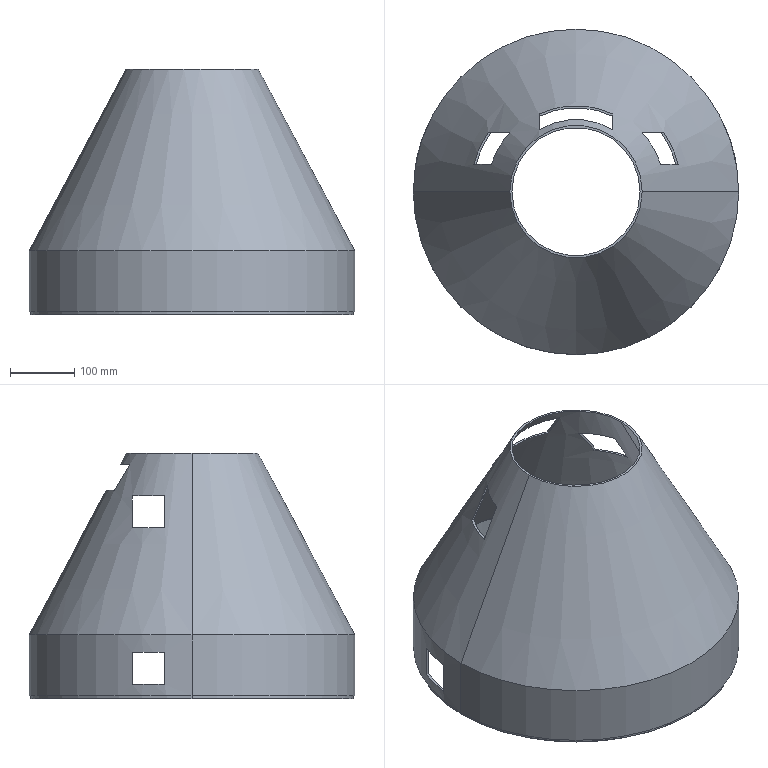Part | SolidWorks | features Cut 2, Extrusion 1, ICE 1, Revolution 1 | 1 solid | 34 faces | box 508 x 508 x 384 mm | volume 1629335 mm3 | plane 24 | cylinder 6 | cone 4 | commonest cylinder face diameters 500 x2 503 x2 508 x2
STEP:
#1=CARTESIAN_POINT('',(-251.5,0.,5.));
#2=VERTEX_POINT('',#1);
#3=CARTESIAN_POINT('',(251.5,0.,5.));
#4=VERTEX_POINT('',#3);
#5=CARTESIAN_POINT('',(0.,0.,5.));
#6=DIRECTION('',(0.,0.,-1.));
#7=DIRECTION('',(-1.,0.,0.));
#8=AXIS2_PLACEMENT_3D('',#5,#6,#7);
#9=CIRCLE('',#8,251.5);
#10=EDGE_CURVE('',#2,#4,#9,.T.);
#11=ORIENTED_EDGE('',*,*,#10,.T.);
#12=CARTESIAN_POINT('',(251.5,0.,0.));
#13=VERTEX_POINT('',#12);
#14=CARTESIAN_POINT('',(251.5,0.,5.));
#15=DIRECTION('',(0.,0.,-1.));
#16=VECTOR('',#15,1000.);
#17=LINE('',#14,#16);
#18=EDGE_CURVE('',#4,#13,#17,.T.);
#19=ORIENTED_EDGE('',*,*,#18,.T.);
#20=CARTESIAN_POINT('',(-251.5,0.,0.));
#21=VERTEX_POINT('',#20);
#22=CARTESIAN_POINT('',(0.,0.,0.));
#23=DIRECTION('',(0.,0.,-1.));
#24=DIRECTION('',(-1.,0.,0.));
#25=AXIS2_PLACEMENT_3D('',#22,#23,#24);
#26=CIRCLE('',#25,251.5);
#27=EDGE_CURVE('',#21,#13,#26,.T.);
#28=ORIENTED_EDGE('',*,*,#27,.F.);
#29=CARTESIAN_POINT('',(-251.5,0.,5.));
#30=DIRECTION('',(0.,0.,-1.));
#31=VECTOR('',#30,1000.);
#32=LINE('',#29,#31);
#33=EDGE_CURVE('',#2,#21,#32,.T.);
#34=ORIENTED_EDGE('',*,*,#33,.F.);
#35=EDGE_LOOP('',(#11,#19,#28,#34));
#36=FACE_OUTER_BOUND('',#35,.T.);
#37=CARTESIAN_POINT('',(0.,0.,5.));
#38=DIRECTION('',(0.,0.,-1.));
#39=DIRECTION('',(-1.,0.,0.));
#40=AXIS2_PLACEMENT_3D('',#37,#38,#39);
#41=CYLINDRICAL_SURFACE('',#40,251.5);
#42=ADVANCED_FACE('',(#36),#41,.T.);
#43=CARTESIAN_POINT('',(100.,0.,384.));
#44=VERTEX_POINT('',#43);
#45=CARTESIAN_POINT('',(-100.,0.,384.));
#46=VERTEX_POINT('',#45);
#47=CARTESIAN_POINT('',(0.,0.,384.));
#48=DIRECTION('',(0.,0.,-1.));
#49=DIRECTION('',(-1.,0.,0.));
#50=AXIS2_PLACEMENT_3D('',#47,#48,#49);
#51=CIRCLE('',#50,100.);
#52=EDGE_CURVE('',#44,#46,#51,.T.);
#53=ORIENTED_EDGE('',*,*,#52,.F.);
#54=CARTESIAN_POINT('',(250.604,0.,100.));
#55=VERTEX_POINT('',#54);
#56=CARTESIAN_POINT('',(250.604,0.,100.));
#57=DIRECTION('',(0.4685,0.,-0.8835));
#58=VECTOR('',#57,1000.);
#59=LINE('',#56,#58);
#60=EDGE_CURVE('',#44,#55,#59,.T.);
#61=ORIENTED_EDGE('',*,*,#60,.T.);
#62=CARTESIAN_POINT('',(-250.604,0.,100.));
#63=VERTEX_POINT('',#62);
#64=CARTESIAN_POINT('',(0.,0.,100.));
#65=DIRECTION('',(0.,0.,-1.));
#66=DIRECTION('',(-1.,0.,0.));
#67=AXIS2_PLACEMENT_3D('',#64,#65,#66);
#68=CIRCLE('',#67,250.604);
#69=EDGE_CURVE('',#55,#63,#68,.T.);
#70=ORIENTED_EDGE('',*,*,#69,.T.);
#71=CARTESIAN_POINT('',(-250.604,0.,100.));
#72=DIRECTION('',(-0.4685,0.,-0.8835));
#73=VECTOR('',#72,1000.);
#74=LINE('',#71,#73);
#75=EDGE_CURVE('',#46,#63,#74,.T.);
#76=ORIENTED_EDGE('',*,*,#75,.F.);
#77=EDGE_LOOP('',(#53,#61,#70,#76));
#78=FACE_OUTER_BOUND('',#77,.T.);
#79=CARTESIAN_POINT('',(0.,0.,100.));
#80=DIRECTION('',(0.,0.,-1.));
#81=DIRECTION('',(-1.,0.,0.));
#82=AXIS2_PLACEMENT_3D('',#79,#80,#81);
#83=CONICAL_SURFACE('',#82,250.604,0.4876);
#84=ADVANCED_FACE('',(#78),#83,.F.);
#85=CARTESIAN_POINT('',(57.407,96.803,366.747));
#86=VERTEX_POINT('',#85);
#87=CARTESIAN_POINT('',(-57.217,96.915,366.747));
#88=VERTEX_POINT('',#87);
#89=CARTESIAN_POINT('',(0.,0.,366.747));
#90=DIRECTION('',(0.,0.,1.));
#91=DIRECTION('',(0.,-1.,0.));
#92=AXIS2_PLACEMENT_3D('',#89,#90,#91);
#93=CIRCLE('',#92,112.545);
#94=EDGE_CURVE('',#86,#88,#93,.T.);
#95=ORIENTED_EDGE('',*,*,#94,.T.);
#96=CARTESIAN_POINT('',(-57.217,121.451,325.81));
#97=VERTEX_POINT('',#96);
#98=CARTESIAN_POINT('',(-57.217,96.915,366.747));
#99=CARTESIAN_POINT('',(-57.217,101.084,359.978));
#100=CARTESIAN_POINT('',(-57.217,105.204,353.175));
#101=CARTESIAN_POINT('',(-57.217,113.376,339.524));
#102=CARTESIAN_POINT('',(-57.217,117.427,332.674));
#103=CARTESIAN_POINT('',(-57.217,121.451,325.81));
#104=B_SPLINE_CURVE_WITH_KNOTS('',3,(#98,#99,#100,#101,#102,#103),.UNSPECIFIED.,.F.,.F.,(4,2,4),(0.4066,0.43,0.4535),.UNSPECIFIED.);
#105=EDGE_CURVE('',#88,#97,#104,.T.);
#106=ORIENTED_EDGE('',*,*,#105,.T.);
#107=CARTESIAN_POINT('',(57.407,121.361,325.81));
#108=VERTEX_POINT('',#107);
#109=CARTESIAN_POINT('',(0.,0.,325.81));
#110=DIRECTION('',(0.,0.,-1.));
#111=DIRECTION('',(0.,1.,0.));
#112=AXIS2_PLACEMENT_3D('',#109,#110,#111);
#113=CIRCLE('',#112,134.254);
#114=EDGE_CURVE('',#97,#108,#113,.T.);
#115=ORIENTED_EDGE('',*,*,#114,.T.);
#116=CARTESIAN_POINT('',(57.407,121.361,325.81));
#117=CARTESIAN_POINT('',(57.407,117.335,332.673));
#118=CARTESIAN_POINT('',(57.407,113.282,339.521));
#119=CARTESIAN_POINT('',(57.407,105.104,353.171));
#120=CARTESIAN_POINT('',(57.407,100.979,359.974));
#121=CARTESIAN_POINT('',(57.407,96.803,366.747));
#122=B_SPLINE_CURVE_WITH_KNOTS('',3,(#116,#117,#118,#119,#120,#121),.UNSPECIFIED.,.F.,.F.,(4,2,4),(0.1407,0.1646,0.1885),.UNSPECIFIED.);
#123=EDGE_CURVE('',#108,#86,#122,.T.);
#124=ORIENTED_EDGE('',*,*,#123,.T.);
#125=EDGE_LOOP('',(#95,#106,#115,#124));
#126=FACE_BOUND('',#125,.T.);
#127=CARTESIAN_POINT('',(159.672,42.9,267.2));
#128=VERTEX_POINT('',#127);
#129=CARTESIAN_POINT('',(132.024,42.9,317.2));
#130=VERTEX_POINT('',#129);
#131=CARTESIAN_POINT('',(159.672,42.9,267.2));
#132=CARTESIAN_POINT('',(150.505,42.9,283.893));
#133=CARTESIAN_POINT('',(141.3,42.9,300.566));
#134=CARTESIAN_POINT('',(132.024,42.9,317.2));
#135=B_SPLINE_CURVE_WITH_KNOTS('',3,(#131,#132,#133,#134),.UNSPECIFIED.,.F.,.F.,(4,4),(0.348,0.4051),.UNSPECIFIED.);
#136=EDGE_CURVE('',#128,#130,#135,.T.);
#137=ORIENTED_EDGE('',*,*,#136,.T.);
#138=CARTESIAN_POINT('',(103.153,92.9,317.2));
#139=VERTEX_POINT('',#138);
#140=CARTESIAN_POINT('',(0.,0.,317.2));
#141=DIRECTION('',(0.,0.,1.));
#142=DIRECTION('',(1.,0.,0.));
#143=AXIS2_PLACEMENT_3D('',#140,#141,#142);
#144=CIRCLE('',#143,138.82);
#145=EDGE_CURVE('',#130,#139,#144,.T.);
#146=ORIENTED_EDGE('',*,*,#145,.T.);
#147=CARTESIAN_POINT('',(136.766,92.9,267.2));
#148=VERTEX_POINT('',#147);
#149=CARTESIAN_POINT('',(103.153,92.9,317.2));
#150=CARTESIAN_POINT('',(108.982,92.9,309.031));
#151=CARTESIAN_POINT('',(114.668,92.9,300.759));
#152=CARTESIAN_POINT('',(125.848,92.9,284.074));
#153=CARTESIAN_POINT('',(131.342,92.9,275.662));
#154=CARTESIAN_POINT('',(136.766,92.9,267.2));
#155=B_SPLINE_CURVE_WITH_KNOTS('',3,(#149,#150,#151,#152,#153,#154),.UNSPECIFIED.,.F.,.F.,(4,2,4),(0.6909,0.7211,0.7513),.UNSPECIFIED.);
#156=EDGE_CURVE('',#139,#148,#155,.T.);
#157=ORIENTED_EDGE('',*,*,#156,.T.);
#158=CARTESIAN_POINT('',(0.,0.,267.2));
#159=DIRECTION('',(0.,0.,-1.));
#160=DIRECTION('',(-1.,0.,0.));
#161=AXIS2_PLACEMENT_3D('',#158,#159,#160);
#162=CIRCLE('',#161,165.334);
#163=EDGE_CURVE('',#148,#128,#162,.T.);
#164=ORIENTED_EDGE('',*,*,#163,.T.);
#165=EDGE_LOOP('',(#137,#146,#157,#164));
#166=FACE_BOUND('',#165,.T.);
#167=CARTESIAN_POINT('',(-136.766,92.9,267.2));
#168=VERTEX_POINT('',#167);
#169=CARTESIAN_POINT('',(-103.153,92.9,317.2));
#170=VERTEX_POINT('',#169);
#171=CARTESIAN_POINT('',(-136.766,92.9,267.2));
#172=CARTESIAN_POINT('',(-131.352,92.9,275.646));
#173=CARTESIAN_POINT('',(-125.865,92.9,284.05));
#174=CARTESIAN_POINT('',(-114.686,92.9,300.732));
#175=CARTESIAN_POINT('',(-108.996,92.9,309.012));
#176=CARTESIAN_POINT('',(-103.153,92.9,317.2));
#177=B_SPLINE_CURVE_WITH_KNOTS('',3,(#171,#172,#173,#174,#175,#176),.UNSPECIFIED.,.F.,.F.,(4,2,4),(0.354,0.384,0.4141),.UNSPECIFIED.);
#178=EDGE_CURVE('',#168,#170,#177,.T.);
#179=ORIENTED_EDGE('',*,*,#178,.T.);
#180=CARTESIAN_POINT('',(-132.024,42.9,317.2));
#181=VERTEX_POINT('',#180);
#182=CARTESIAN_POINT('',(0.,0.,317.2));
#183=DIRECTION('',(0.,0.,1.));
#184=DIRECTION('',(1.,0.,0.));
#185=AXIS2_PLACEMENT_3D('',#182,#183,#184);
#186=CIRCLE('',#185,138.82);
#187=EDGE_CURVE('',#170,#181,#186,.T.);
#188=ORIENTED_EDGE('',*,*,#187,.T.);
#189=CARTESIAN_POINT('',(-159.672,42.9,267.2));
#190=VERTEX_POINT('',#189);
#191=CARTESIAN_POINT('',(-132.024,42.9,317.2));
#192=CARTESIAN_POINT('',(-141.299,42.9,300.567));
#193=CARTESIAN_POINT('',(-150.505,42.9,283.895));
#194=CARTESIAN_POINT('',(-159.672,42.9,267.2));
#195=B_SPLINE_CURVE_WITH_KNOTS('',3,(#191,#192,#193,#194),.UNSPECIFIED.,.F.,.F.,(4,4),(0.8629,0.9203),.UNSPECIFIED.);
#196=EDGE_CURVE('',#181,#190,#195,.T.);
#197=ORIENTED_EDGE('',*,*,#196,.T.);
#198=CARTESIAN_POINT('',(0.,0.,267.2));
#199=DIRECTION('',(0.,0.,-1.));
#200=DIRECTION('',(-1.,0.,0.));
#201=AXIS2_PLACEMENT_3D('',#198,#199,#200);
#202=CIRCLE('',#201,165.334);
#203=EDGE_CURVE('',#190,#168,#202,.T.);
#204=ORIENTED_EDGE('',*,*,#203,.T.);
#205=EDGE_LOOP('',(#179,#188,#197,#204));
#206=FACE_BOUND('',#205,.T.);
#207=CARTESIAN_POINT('',(-103.396,0.,384.));
#208=VERTEX_POINT('',#207);
#209=CARTESIAN_POINT('',(103.396,0.,384.));
#210=VERTEX_POINT('',#209);
#211=CARTESIAN_POINT('',(0.,0.,384.));
#212=DIRECTION('',(0.,0.,-1.));
#213=DIRECTION('',(-1.,0.,0.));
#214=AXIS2_PLACEMENT_3D('',#211,#212,#213);
#215=CIRCLE('',#214,103.396);
#216=EDGE_CURVE('',#208,#210,#215,.T.);
#217=ORIENTED_EDGE('',*,*,#216,.T.);
#218=CARTESIAN_POINT('',(254.,0.,100.));
#219=VERTEX_POINT('',#218);
#220=CARTESIAN_POINT('',(103.396,0.,384.));
#221=DIRECTION('',(0.4685,0.,-0.8835));
#222=VECTOR('',#221,1000.);
#223=LINE('',#220,#222);
#224=EDGE_CURVE('',#210,#219,#223,.T.);
#225=ORIENTED_EDGE('',*,*,#224,.T.);
#226=CARTESIAN_POINT('',(-254.,0.,100.));
#227=VERTEX_POINT('',#226);
#228=CARTESIAN_POINT('',(0.,0.,100.));
#229=DIRECTION('',(0.,0.,1.));
#230=DIRECTION('',(1.,0.,0.));
#231=AXIS2_PLACEMENT_3D('',#228,#229,#230);
#232=CIRCLE('',#231,254.);
#233=EDGE_CURVE('',#219,#227,#232,.T.);
#234=ORIENTED_EDGE('',*,*,#233,.T.);
#235=CARTESIAN_POINT('',(-103.396,0.,384.));
#236=DIRECTION('',(-0.4685,0.,-0.8835));
#237=VECTOR('',#236,1000.);
#238=LINE('',#235,#237);
#239=EDGE_CURVE('',#208,#227,#238,.T.);
#240=ORIENTED_EDGE('',*,*,#239,.F.);
#241=EDGE_LOOP('',(#217,#225,#234,#240));
#242=FACE_OUTER_BOUND('',#241,.T.);
#243=CARTESIAN_POINT('',(0.,0.,384.));
#244=DIRECTION('',(0.,0.,-1.));
#245=DIRECTION('',(-1.,0.,0.));
#246=AXIS2_PLACEMENT_3D('',#243,#244,#245);
#247=CONICAL_SURFACE('',#246,103.396,0.4876);
#248=ADVANCED_FACE('',(#126,#166,#206,#242),#247,.T.);
#249=CARTESIAN_POINT('',(-250.,0.,100.));
#250=VERTEX_POINT('',#249);
#251=CARTESIAN_POINT('',(250.,0.,100.));
#252=VERTEX_POINT('',#251);
#253=CARTESIAN_POINT('',(0.,0.,100.));
#254=DIRECTION('',(0.,0.,1.));
#255=DIRECTION('',(1.,0.,0.));
#256=AXIS2_PLACEMENT_3D('',#253,#254,#255);
#257=CIRCLE('',#256,250.);
#258=EDGE_CURVE('',#250,#252,#257,.T.);
#259=ORIENTED_EDGE('',*,*,#258,.T.);
#260=CARTESIAN_POINT('',(250.,0.,0.));
#261=VERTEX_POINT('',#260);
#262=CARTESIAN_POINT('',(250.,0.,100.));
#263=DIRECTION('',(0.,0.,-1.));
#264=VECTOR('',#263,1000.);
#265=LINE('',#262,#264);
#266=EDGE_CURVE('',#252,#261,#265,.T.);
#267=ORIENTED_EDGE('',*,*,#266,.T.);
#268=CARTESIAN_POINT('',(-250.,0.,0.));
#269=VERTEX_POINT('',#268);
#270=CARTESIAN_POINT('',(0.,0.,0.));
#271=DIRECTION('',(0.,0.,1.));
#272=DIRECTION('',(1.,0.,0.));
#273=AXIS2_PLACEMENT_3D('',#270,#271,#272);
#274=CIRCLE('',#273,250.);
#275=EDGE_CURVE('',#269,#261,#274,.T.);
#276=ORIENTED_EDGE('',*,*,#275,.F.);
#277=CARTESIAN_POINT('',(-250.,0.,100.));
#278=DIRECTION('',(0.,0.,-1.));
#279=VECTOR('',#278,1000.);
#280=LINE('',#277,#279);
#281=EDGE_CURVE('',#250,#269,#280,.T.);
#282=ORIENTED_EDGE('',*,*,#281,.F.);
#283=EDGE_LOOP('',(#259,#267,#276,#282));
#284=FACE_OUTER_BOUND('',#283,.T.);
#285=CARTESIAN_POINT('',(0.,0.,100.));
#286=DIRECTION('',(0.,0.,-1.));
#287=DIRECTION('',(-1.,0.,0.));
#288=AXIS2_PLACEMENT_3D('',#285,#286,#287);
#289=CYLINDRICAL_SURFACE('',#288,250.);
#290=ADVANCED_FACE('',(#284),#289,.F.);
#291=CARTESIAN_POINT('',(250.351,42.9,22.8));
#292=VERTEX_POINT('',#291);
#293=CARTESIAN_POINT('',(250.351,42.9,72.8));
#294=VERTEX_POINT('',#293);
#295=CARTESIAN_POINT('',(250.351,42.9,100.));
#296=DIRECTION('',(0.,0.,1.));
#297=VECTOR('',#296,1000.);
#298=LINE('',#295,#297);
#299=EDGE_CURVE('',#292,#294,#298,.T.);
#300=ORIENTED_EDGE('',*,*,#299,.T.);
#301=CARTESIAN_POINT('',(236.401,92.9,72.8));
#302=VERTEX_POINT('',#301);
#303=CARTESIAN_POINT('',(0.,0.,72.8));
#304=DIRECTION('',(0.,0.,1.));
#305=DIRECTION('',(1.,0.,0.));
#306=AXIS2_PLACEMENT_3D('',#303,#304,#305);
#307=CIRCLE('',#306,254.);
#308=EDGE_CURVE('',#294,#302,#307,.T.);
#309=ORIENTED_EDGE('',*,*,#308,.T.);
#310=CARTESIAN_POINT('',(236.401,92.9,22.8));
#311=VERTEX_POINT('',#310);
#312=CARTESIAN_POINT('',(236.401,92.9,100.));
#313=DIRECTION('',(0.,0.,-1.));
#314=VECTOR('',#313,1000.);
#315=LINE('',#312,#314);
#316=EDGE_CURVE('',#302,#311,#315,.T.);
#317=ORIENTED_EDGE('',*,*,#316,.T.);
#318=CARTESIAN_POINT('',(0.,0.,22.8));
#319=DIRECTION('',(0.,0.,-1.));
#320=DIRECTION('',(-1.,0.,0.));
#321=AXIS2_PLACEMENT_3D('',#318,#319,#320);
#322=CIRCLE('',#321,254.);
#323=EDGE_CURVE('',#311,#292,#322,.T.);
#324=ORIENTED_EDGE('',*,*,#323,.T.);
#325=EDGE_LOOP('',(#300,#309,#317,#324));
#326=FACE_BOUND('',#325,.T.);
#327=CARTESIAN_POINT('',(-236.401,92.9,22.8));
#328=VERTEX_POINT('',#327);
#329=CARTESIAN_POINT('',(-236.401,92.9,72.8));
#330=VERTEX_POINT('',#329);
#331=CARTESIAN_POINT('',(-236.401,92.9,100.));
#332=DIRECTION('',(0.,0.,1.));
#333=VECTOR('',#332,1000.);
#334=LINE('',#331,#333);
#335=EDGE_CURVE('',#328,#330,#334,.T.);
#336=ORIENTED_EDGE('',*,*,#335,.T.);
#337=CARTESIAN_POINT('',(-250.351,42.9,72.8));
#338=VERTEX_POINT('',#337);
#339=CARTESIAN_POINT('',(0.,0.,72.8));
#340=DIRECTION('',(0.,0.,1.));
#341=DIRECTION('',(1.,0.,0.));
#342=AXIS2_PLACEMENT_3D('',#339,#340,#341);
#343=CIRCLE('',#342,254.);
#344=EDGE_CURVE('',#330,#338,#343,.T.);
#345=ORIENTED_EDGE('',*,*,#344,.T.);
#346=CARTESIAN_POINT('',(-250.351,42.9,22.8));
#347=VERTEX_POINT('',#346);
#348=CARTESIAN_POINT('',(-250.351,42.9,100.));
#349=DIRECTION('',(0.,0.,-1.));
#350=VECTOR('',#349,1000.);
#351=LINE('',#348,#350);
#352=EDGE_CURVE('',#338,#347,#351,.T.);
#353=ORIENTED_EDGE('',*,*,#352,.T.);
#354=CARTESIAN_POINT('',(0.,0.,22.8));
#355=DIRECTION('',(0.,0.,-1.));
#356=DIRECTION('',(-1.,0.,0.));
#357=AXIS2_PLACEMENT_3D('',#354,#355,#356);
#358=CIRCLE('',#357,254.);
#359=EDGE_CURVE('',#347,#328,#358,.T.);
#360=ORIENTED_EDGE('',*,*,#359,.T.);
#361=EDGE_LOOP('',(#336,#345,#353,#360));
#362=FACE_BOUND('',#361,.T.);
#363=ORIENTED_EDGE('',*,*,#233,.F.);
#364=CARTESIAN_POINT('',(254.,0.,5.));
#365=VERTEX_POINT('',#364);
#366=CARTESIAN_POINT('',(254.,0.,100.));
#367=DIRECTION('',(0.,0.,-1.));
#368=VECTOR('',#367,1000.);
#369=LINE('',#366,#368);
#370=EDGE_CURVE('',#219,#365,#369,.T.);
#371=ORIENTED_EDGE('',*,*,#370,.T.);
#372=CARTESIAN_POINT('',(-254.,0.,5.));
#373=VERTEX_POINT('',#372);
#374=CARTESIAN_POINT('',(0.,0.,5.));
#375=DIRECTION('',(0.,0.,-1.));
#376=DIRECTION('',(-1.,0.,0.));
#377=AXIS2_PLACEMENT_3D('',#374,#375,#376);
#378=CIRCLE('',#377,254.);
#379=EDGE_CURVE('',#373,#365,#378,.T.);
#380=ORIENTED_EDGE('',*,*,#379,.F.);
#381=CARTESIAN_POINT('',(-254.,0.,100.));
#382=DIRECTION('',(0.,0.,-1.));
#383=VECTOR('',#382,1000.);
#384=LINE('',#381,#383);
#385=EDGE_CURVE('',#227,#373,#384,.T.);
#386=ORIENTED_EDGE('',*,*,#385,.F.);
#387=EDGE_LOOP('',(#363,#371,#380,#386));
#388=FACE_OUTER_BOUND('',#387,.T.);
#389=CARTESIAN_POINT('',(0.,0.,100.));
#390=DIRECTION('',(0.,0.,-1.));
#391=DIRECTION('',(-1.,0.,0.));
#392=AXIS2_PLACEMENT_3D('',#389,#390,#391);
#393=CYLINDRICAL_SURFACE('',#392,254.);
#394=ADVANCED_FACE('',(#326,#362,#388),#393,.T.);
#395=ORIENTED_EDGE('',*,*,#275,.T.);
#396=CARTESIAN_POINT('',(0.,0.,0.));
#397=DIRECTION('',(0.,0.,1.));
#398=DIRECTION('',(1.,0.,0.));
#399=AXIS2_PLACEMENT_3D('',#396,#397,#398);
#400=CIRCLE('',#399,250.);
#401=EDGE_CURVE('',#261,#269,#400,.T.);
#402=ORIENTED_EDGE('',*,*,#401,.T.);
#403=EDGE_LOOP('',(#395,#402));
#404=FACE_BOUND('',#403,.T.);
#405=ORIENTED_EDGE('',*,*,#27,.T.);
#406=CARTESIAN_POINT('',(0.,0.,0.));
#407=DIRECTION('',(0.,0.,-1.));
#408=DIRECTION('',(-1.,0.,0.));
#409=AXIS2_PLACEMENT_3D('',#406,#407,#408);
#410=CIRCLE('',#409,251.5);
#411=EDGE_CURVE('',#13,#21,#410,.T.);
#412=ORIENTED_EDGE('',*,*,#411,.T.);
#413=EDGE_LOOP('',(#405,#412));
#414=FACE_OUTER_BOUND('',#413,.T.);
#415=CARTESIAN_POINT('',(0.,0.,0.));
#416=DIRECTION('',(0.,0.,1.));
#417=DIRECTION('',(1.,0.,0.));
#418=AXIS2_PLACEMENT_3D('',#415,#416,#417);
#419=PLANE('',#418);
#420=ADVANCED_FACE('',(#404,#414),#419,.F.);
#421=ORIENTED_EDGE('',*,*,#370,.F.);
#422=CARTESIAN_POINT('',(0.,0.,100.));
#423=DIRECTION('',(0.,0.,1.));
#424=DIRECTION('',(1.,0.,0.));
#425=AXIS2_PLACEMENT_3D('',#422,#423,#424);
#426=CIRCLE('',#425,254.);
#427=EDGE_CURVE('',#227,#219,#426,.T.);
#428=ORIENTED_EDGE('',*,*,#427,.F.);
#429=ORIENTED_EDGE('',*,*,#385,.T.);
#430=CARTESIAN_POINT('',(0.,0.,5.));
#431=DIRECTION('',(0.,0.,-1.));
#432=DIRECTION('',(-1.,0.,0.));
#433=AXIS2_PLACEMENT_3D('',#430,#431,#432);
#434=CIRCLE('',#433,254.);
#435=EDGE_CURVE('',#365,#373,#434,.T.);
#436=ORIENTED_EDGE('',*,*,#435,.F.);
#437=EDGE_LOOP('',(#421,#428,#429,#436));
#438=FACE_OUTER_BOUND('',#437,.T.);
#439=CARTESIAN_POINT('',(0.,0.,100.));
#440=DIRECTION('',(0.,0.,-1.));
#441=DIRECTION('',(-1.,0.,0.));
#442=AXIS2_PLACEMENT_3D('',#439,#440,#441);
#443=CYLINDRICAL_SURFACE('',#442,254.);
#444=ADVANCED_FACE('',(#438),#443,.T.);
#445=ORIENTED_EDGE('',*,*,#258,.F.);
#446=CARTESIAN_POINT('',(0.,0.,100.));
#447=DIRECTION('',(0.,0.,1.));
#448=DIRECTION('',(1.,0.,0.));
#449=AXIS2_PLACEMENT_3D('',#446,#447,#448);
#450=CIRCLE('',#449,250.);
#451=EDGE_CURVE('',#252,#250,#450,.T.);
#452=ORIENTED_EDGE('',*,*,#451,.F.);
#453=EDGE_LOOP('',(#445,#452));
#454=FACE_BOUND('',#453,.T.);
#455=CARTESIAN_POINT('',(0.,0.,100.));
#456=DIRECTION('',(0.,0.,-1.));
#457=DIRECTION('',(-1.,0.,0.));
#458=AXIS2_PLACEMENT_3D('',#455,#456,#457);
#459=CIRCLE('',#458,250.604);
#460=EDGE_CURVE('',#63,#55,#459,.T.);
#461=ORIENTED_EDGE('',*,*,#460,.F.);
#462=ORIENTED_EDGE('',*,*,#69,.F.);
#463=EDGE_LOOP('',(#461,#462));
#464=FACE_OUTER_BOUND('',#463,.T.);
#465=CARTESIAN_POINT('',(0.,0.,100.));
#466=DIRECTION('',(0.,0.,1.));
#467=DIRECTION('',(1.,0.,0.));
#468=AXIS2_PLACEMENT_3D('',#465,#466,#467);
#469=PLANE('',#468);
#470=ADVANCED_FACE('',(#454,#464),#469,.T.);
#471=ORIENTED_EDGE('',*,*,#266,.F.);
#472=ORIENTED_EDGE('',*,*,#451,.T.);
#473=ORIENTED_EDGE('',*,*,#281,.T.);
#474=ORIENTED_EDGE('',*,*,#401,.F.);
#475=EDGE_LOOP('',(#471,#472,#473,#474));
#476=FACE_OUTER_BOUND('',#475,.T.);
#477=CARTESIAN_POINT('',(-232.098,92.9,72.8));
#478=VERTEX_POINT('',#477);
#479=CARTESIAN_POINT('',(-246.292,42.9,72.8));
#480=VERTEX_POINT('',#479);
#481=CARTESIAN_POINT('',(0.,0.,72.8));
#482=DIRECTION('',(0.,0.,1.));
#483=DIRECTION('',(1.,0.,0.));
#484=AXIS2_PLACEMENT_3D('',#481,#482,#483);
#485=CIRCLE('',#484,250.);
#486=EDGE_CURVE('',#478,#480,#485,.T.);
#487=ORIENTED_EDGE('',*,*,#486,.F.);
#488=CARTESIAN_POINT('',(-232.098,92.9,22.8));
#489=VERTEX_POINT('',#488);
#490=CARTESIAN_POINT('',(-232.098,92.9,100.));
#491=DIRECTION('',(0.,0.,1.));
#492=VECTOR('',#491,1000.);
#493=LINE('',#490,#492);
#494=EDGE_CURVE('',#489,#478,#493,.T.);
#495=ORIENTED_EDGE('',*,*,#494,.F.);
#496=CARTESIAN_POINT('',(-246.292,42.9,22.8));
#497=VERTEX_POINT('',#496);
#498=CARTESIAN_POINT('',(0.,0.,22.8));
#499=DIRECTION('',(0.,0.,-1.));
#500=DIRECTION('',(-1.,0.,0.));
#501=AXIS2_PLACEMENT_3D('',#498,#499,#500);
#502=CIRCLE('',#501,250.);
#503=EDGE_CURVE('',#497,#489,#502,.T.);
#504=ORIENTED_EDGE('',*,*,#503,.F.);
#505=CARTESIAN_POINT('',(-246.292,42.9,100.));
#506=DIRECTION('',(0.,0.,-1.));
#507=VECTOR('',#506,1000.);
#508=LINE('',#505,#507);
#509=EDGE_CURVE('',#480,#497,#508,.T.);
#510=ORIENTED_EDGE('',*,*,#509,.F.);
#511=EDGE_LOOP('',(#487,#495,#504,#510));
#512=FACE_BOUND('',#511,.T.);
#513=CARTESIAN_POINT('',(246.292,42.9,72.8));
#514=VERTEX_POINT('',#513);
#515=CARTESIAN_POINT('',(232.098,92.9,72.8));
#516=VERTEX_POINT('',#515);
#517=CARTESIAN_POINT('',(0.,0.,72.8));
#518=DIRECTION('',(0.,0.,1.));
#519=DIRECTION('',(1.,0.,0.));
#520=AXIS2_PLACEMENT_3D('',#517,#518,#519);
#521=CIRCLE('',#520,250.);
#522=EDGE_CURVE('',#514,#516,#521,.T.);
#523=ORIENTED_EDGE('',*,*,#522,.F.);
#524=CARTESIAN_POINT('',(246.292,42.9,22.8));
#525=VERTEX_POINT('',#524);
#526=CARTESIAN_POINT('',(246.292,42.9,100.));
#527=DIRECTION('',(0.,0.,1.));
#528=VECTOR('',#527,1000.);
#529=LINE('',#526,#528);
#530=EDGE_CURVE('',#525,#514,#529,.T.);
#531=ORIENTED_EDGE('',*,*,#530,.F.);
#532=CARTESIAN_POINT('',(232.098,92.9,22.8));
#533=VERTEX_POINT('',#532);
#534=CARTESIAN_POINT('',(0.,0.,22.8));
#535=DIRECTION('',(0.,0.,-1.));
#536=DIRECTION('',(-1.,0.,0.));
#537=AXIS2_PLACEMENT_3D('',#534,#535,#536);
#538=CIRCLE('',#537,250.);
#539=EDGE_CURVE('',#533,#525,#538,.T.);
#540=ORIENTED_EDGE('',*,*,#539,.F.);
#541=CARTESIAN_POINT('',(232.098,92.9,100.));
#542=DIRECTION('',(0.,0.,-1.));
#543=VECTOR('',#542,1000.);
#544=LINE('',#541,#543);
#545=EDGE_CURVE('',#516,#533,#544,.T.);
#546=ORIENTED_EDGE('',*,*,#545,.F.);
#547=EDGE_LOOP('',(#523,#531,#540,#546));
#548=FACE_BOUND('',#547,.T.);
#549=CARTESIAN_POINT('',(0.,0.,100.));
#550=DIRECTION('',(0.,0.,-1.));
#551=DIRECTION('',(-1.,0.,0.));
#552=AXIS2_PLACEMENT_3D('',#549,#550,#551);
#553=CYLINDRICAL_SURFACE('',#552,250.);
#554=ADVANCED_FACE('',(#476,#512,#548),#553,.F.);
#555=ORIENTED_EDGE('',*,*,#224,.F.);
#556=CARTESIAN_POINT('',(0.,0.,384.));
#557=DIRECTION('',(0.,0.,-1.));
#558=DIRECTION('',(-1.,0.,0.));
#559=AXIS2_PLACEMENT_3D('',#556,#557,#558);
#560=CIRCLE('',#559,103.396);
#561=EDGE_CURVE('',#210,#208,#560,.T.);
#562=ORIENTED_EDGE('',*,*,#561,.T.);
#563=ORIENTED_EDGE('',*,*,#239,.T.);
#564=ORIENTED_EDGE('',*,*,#427,.T.);
#565=EDGE_LOOP('',(#555,#562,#563,#564));
#566=FACE_OUTER_BOUND('',#565,.T.);
#567=CARTESIAN_POINT('',(0.,0.,384.));
#568=DIRECTION('',(0.,0.,-1.));
#569=DIRECTION('',(-1.,0.,0.));
#570=AXIS2_PLACEMENT_3D('',#567,#568,#569);
#571=CONICAL_SURFACE('',#570,103.396,0.4876);
#572=ADVANCED_FACE('',(#566),#571,.T.);
#573=ORIENTED_EDGE('',*,*,#216,.F.);
#574=ORIENTED_EDGE('',*,*,#561,.F.);
#575=EDGE_LOOP('',(#573,#574));
#576=FACE_OUTER_BOUND('',#575,.T.);
#577=CARTESIAN_POINT('',(0.,0.,384.));
#578=DIRECTION('',(0.,0.,-1.));
#579=DIRECTION('',(-1.,0.,0.));
#580=AXIS2_PLACEMENT_3D('',#577,#578,#579);
#581=CIRCLE('',#580,100.);
#582=EDGE_CURVE('',#46,#44,#581,.T.);
#583=ORIENTED_EDGE('',*,*,#582,.T.);
#584=ORIENTED_EDGE('',*,*,#52,.T.);
#585=EDGE_LOOP('',(#583,#584));
#586=FACE_BOUND('',#585,.T.);
#587=CARTESIAN_POINT('',(100.,0.,384.));
#588=DIRECTION('',(0.,0.,-1.));
#589=DIRECTION('',(-1.,0.,0.));
#590=AXIS2_PLACEMENT_3D('',#587,#588,#589);
#591=PLANE('',#590);
#592=ADVANCED_FACE('',(#576,#586),#591,.F.);
#593=ORIENTED_EDGE('',*,*,#60,.F.);
#594=ORIENTED_EDGE('',*,*,#582,.F.);
#595=ORIENTED_EDGE('',*,*,#75,.T.);
#596=ORIENTED_EDGE('',*,*,#460,.T.);
#597=EDGE_LOOP('',(#593,#594,#595,#596));
#598=FACE_OUTER_BOUND('',#597,.T.);
#599=CARTESIAN_POINT('',(57.407,117.594,325.81));
#600=VERTEX_POINT('',#599);
#601=CARTESIAN_POINT('',(-57.217,117.686,325.81));
#602=VERTEX_POINT('',#601);
#603=CARTESIAN_POINT('',(0.,0.,325.81));
#604=DIRECTION('',(0.,0.,1.));
#605=DIRECTION('',(0.,1.,0.));
#606=AXIS2_PLACEMENT_3D('',#603,#604,#605);
#607=CIRCLE('',#606,130.858);
#608=EDGE_CURVE('',#600,#602,#607,.T.);
#609=ORIENTED_EDGE('',*,*,#608,.T.);
#610=CARTESIAN_POINT('',(-57.217,92.95,366.747));
#611=VERTEX_POINT('',#610);
#612=CARTESIAN_POINT('',(-57.217,117.686,325.81));
#613=CARTESIAN_POINT('',(-57.217,113.637,332.678));
#614=CARTESIAN_POINT('',(-57.217,109.558,339.527));
#615=CARTESIAN_POINT('',(-57.217,101.322,353.178));
#616=CARTESIAN_POINT('',(-57.217,97.164,359.98));
#617=CARTESIAN_POINT('',(-57.217,92.95,366.747));
#618=B_SPLINE_CURVE_WITH_KNOTS('',3,(#612,#613,#614,#615,#616,#617),.UNSPECIFIED.,.F.,.F.,(4,2,4),(0.1408,0.1647,0.1886),.UNSPECIFIED.);
#619=EDGE_CURVE('',#602,#611,#618,.T.);
#620=ORIENTED_EDGE('',*,*,#619,.T.);
#621=CARTESIAN_POINT('',(57.407,92.833,366.747));
#622=VERTEX_POINT('',#621);
#623=CARTESIAN_POINT('',(0.,0.,366.747));
#624=DIRECTION('',(0.,0.,-1.));
#625=DIRECTION('',(0.,-1.,0.));
#626=AXIS2_PLACEMENT_3D('',#623,#624,#625);
#627=CIRCLE('',#626,109.149);
#628=EDGE_CURVE('',#611,#622,#627,.T.);
#629=ORIENTED_EDGE('',*,*,#628,.T.);
#630=CARTESIAN_POINT('',(57.407,92.833,366.747));
#631=CARTESIAN_POINT('',(57.407,97.05,359.985));
#632=CARTESIAN_POINT('',(57.407,101.211,353.185));
#633=CARTESIAN_POINT('',(57.407,109.455,339.533));
#634=CARTESIAN_POINT('',(57.407,113.539,332.681));
#635=CARTESIAN_POINT('',(57.407,117.594,325.81));
#636=B_SPLINE_CURVE_WITH_KNOTS('',3,(#630,#631,#632,#633,#634,#635),.UNSPECIFIED.,.F.,.F.,(4,2,4),(0.3985,0.422,0.4456),.UNSPECIFIED.);
#637=EDGE_CURVE('',#622,#600,#636,.T.);
#638=ORIENTED_EDGE('',*,*,#637,.T.);
#639=EDGE_LOOP('',(#609,#620,#629,#638));
#640=FACE_BOUND('',#639,.T.);
#641=CARTESIAN_POINT('',(-156.153,42.9,267.2));
#642=VERTEX_POINT('',#641);
#643=CARTESIAN_POINT('',(-128.449,42.9,317.2));
#644=VERTEX_POINT('',#643);
#645=CARTESIAN_POINT('',(-156.153,42.9,267.2));
#646=CARTESIAN_POINT('',(-146.971,42.9,283.895));
#647=CARTESIAN_POINT('',(-137.748,42.9,300.568));
#648=CARTESIAN_POINT('',(-128.449,42.9,317.2));
#649=B_SPLINE_CURVE_WITH_KNOTS('',3,(#645,#646,#647,#648),.UNSPECIFIED.,.F.,.F.,(4,4),(0.3435,0.4006),.UNSPECIFIED.);
#650=EDGE_CURVE('',#642,#644,#649,.T.);
#651=ORIENTED_EDGE('',*,*,#650,.T.);
#652=CARTESIAN_POINT('',(-98.535,92.9,317.2));
#653=VERTEX_POINT('',#652);
#654=CARTESIAN_POINT('',(0.,0.,317.2));
#655=DIRECTION('',(0.,0.,-1.));
#656=DIRECTION('',(1.,0.,0.));
#657=AXIS2_PLACEMENT_3D('',#654,#655,#656);
#658=CIRCLE('',#657,135.424);
#659=EDGE_CURVE('',#644,#653,#658,.T.);
#660=ORIENTED_EDGE('',*,*,#659,.T.);
#661=CARTESIAN_POINT('',(-132.641,92.9,267.2));
#662=VERTEX_POINT('',#661);
#663=CARTESIAN_POINT('',(-98.535,92.9,317.2));
#664=CARTESIAN_POINT('',(-104.489,92.9,309.031));
#665=CARTESIAN_POINT('',(-110.27,92.9,300.757));
#666=CARTESIAN_POINT('',(-121.609,92.9,284.072));
#667=CARTESIAN_POINT('',(-127.164,92.9,275.66));
#668=CARTESIAN_POINT('',(-132.641,92.9,267.2));
#669=B_SPLINE_CURVE_WITH_KNOTS('',3,(#663,#664,#665,#666,#667,#668),.UNSPECIFIED.,.F.,.F.,(4,2,4),(0.6709,0.7012,0.7315),.UNSPECIFIED.);
#670=EDGE_CURVE('',#653,#662,#669,.T.);
#671=ORIENTED_EDGE('',*,*,#670,.T.);
#672=CARTESIAN_POINT('',(0.,0.,267.2));
#673=DIRECTION('',(0.,0.,1.));
#674=DIRECTION('',(-1.,0.,0.));
#675=AXIS2_PLACEMENT_3D('',#672,#673,#674);
#676=CIRCLE('',#675,161.939);
#677=EDGE_CURVE('',#662,#642,#676,.T.);
#678=ORIENTED_EDGE('',*,*,#677,.T.);
#679=EDGE_LOOP('',(#651,#660,#671,#678));
#680=FACE_BOUND('',#679,.T.);
#681=CARTESIAN_POINT('',(132.641,92.9,267.2));
#682=VERTEX_POINT('',#681);
#683=CARTESIAN_POINT('',(98.535,92.9,317.2));
#684=VERTEX_POINT('',#683);
#685=CARTESIAN_POINT('',(132.641,92.9,267.2));
#686=CARTESIAN_POINT('',(127.165,92.9,275.659));
#687=CARTESIAN_POINT('',(121.609,92.9,284.071));
#688=CARTESIAN_POINT('',(110.271,92.9,300.756));
#689=CARTESIAN_POINT('',(104.489,92.9,309.03));
#690=CARTESIAN_POINT('',(98.535,92.9,317.2));
#691=B_SPLINE_CURVE_WITH_KNOTS('',3,(#685,#686,#687,#688,#689,#690),.UNSPECIFIED.,.F.,.F.,(4,2,4),(0.3496,0.3798,0.4101),.UNSPECIFIED.);
#692=EDGE_CURVE('',#682,#684,#691,.T.);
#693=ORIENTED_EDGE('',*,*,#692,.T.);
#694=CARTESIAN_POINT('',(128.449,42.9,317.2));
#695=VERTEX_POINT('',#694);
#696=CARTESIAN_POINT('',(0.,0.,317.2));
#697=DIRECTION('',(0.,0.,-1.));
#698=DIRECTION('',(1.,0.,0.));
#699=AXIS2_PLACEMENT_3D('',#696,#697,#698);
#700=CIRCLE('',#699,135.424);
#701=EDGE_CURVE('',#684,#695,#700,.T.);
#702=ORIENTED_EDGE('',*,*,#701,.T.);
#703=CARTESIAN_POINT('',(156.153,42.9,267.2));
#704=VERTEX_POINT('',#703);
#705=CARTESIAN_POINT('',(128.449,42.9,317.2));
#706=CARTESIAN_POINT('',(137.747,42.9,300.57));
#707=CARTESIAN_POINT('',(146.971,42.9,283.897));
#708=CARTESIAN_POINT('',(156.153,42.9,267.2));
#709=B_SPLINE_CURVE_WITH_KNOTS('',3,(#705,#706,#707,#708),.UNSPECIFIED.,.F.,.F.,(4,4),(0.8436,0.9011),.UNSPECIFIED.);
#710=EDGE_CURVE('',#695,#704,#709,.T.);
#711=ORIENTED_EDGE('',*,*,#710,.T.);
#712=CARTESIAN_POINT('',(0.,0.,267.2));
#713=DIRECTION('',(0.,0.,1.));
#714=DIRECTION('',(-1.,0.,0.));
#715=AXIS2_PLACEMENT_3D('',#712,#713,#714);
#716=CIRCLE('',#715,161.939);
#717=EDGE_CURVE('',#704,#682,#716,.T.);
#718=ORIENTED_EDGE('',*,*,#717,.T.);
#719=EDGE_LOOP('',(#693,#702,#711,#718));
#720=FACE_BOUND('',#719,.T.);
#721=CARTESIAN_POINT('',(0.,0.,100.));
#722=DIRECTION('',(0.,0.,-1.));
#723=DIRECTION('',(-1.,0.,0.));
#724=AXIS2_PLACEMENT_3D('',#721,#722,#723);
#725=CONICAL_SURFACE('',#724,250.604,0.4876);
#726=ADVANCED_FACE('',(#598,#640,#680,#720),#725,.F.);
#727=CARTESIAN_POINT('',(-500.,42.9,22.8));
#728=DIRECTION('',(1.,0.,0.));
#729=VECTOR('',#728,1000.);
#730=LINE('',#727,#729);
#731=EDGE_CURVE('',#525,#292,#730,.T.);
#732=ORIENTED_EDGE('',*,*,#731,.F.);
#733=ORIENTED_EDGE('',*,*,#530,.T.);
#734=CARTESIAN_POINT('',(-500.,42.9,72.8));
#735=DIRECTION('',(1.,0.,0.));
#736=VECTOR('',#735,1000.);
#737=LINE('',#734,#736);
#738=EDGE_CURVE('',#514,#294,#737,.T.);
#739=ORIENTED_EDGE('',*,*,#738,.T.);
#740=ORIENTED_EDGE('',*,*,#299,.F.);
#741=EDGE_LOOP('',(#732,#733,#739,#740));
#742=FACE_OUTER_BOUND('',#741,.T.);
#743=CARTESIAN_POINT('',(-500.,42.9,72.8));
#744=DIRECTION('',(0.,-1.,0.));
#745=DIRECTION('',(0.,0.,-1.));
#746=AXIS2_PLACEMENT_3D('',#743,#744,#745);
#747=PLANE('',#746);
#748=ADVANCED_FACE('',(#742),#747,.F.);
#749=CARTESIAN_POINT('',(-500.,92.9,22.8));
#750=DIRECTION('',(1.,0.,0.));
#751=VECTOR('',#750,1000.);
#752=LINE('',#749,#751);
#753=EDGE_CURVE('',#533,#311,#752,.T.);
#754=ORIENTED_EDGE('',*,*,#753,.F.);
#755=ORIENTED_EDGE('',*,*,#539,.T.);
#756=ORIENTED_EDGE('',*,*,#731,.T.);
#757=ORIENTED_EDGE('',*,*,#323,.F.);
#758=EDGE_LOOP('',(#754,#755,#756,#757));
#759=FACE_OUTER_BOUND('',#758,.T.);
#760=CARTESIAN_POINT('',(-500.,92.9,22.8));
#761=DIRECTION('',(0.,0.,-1.));
#762=DIRECTION('',(-1.,0.,0.));
#763=AXIS2_PLACEMENT_3D('',#760,#761,#762);
#764=PLANE('',#763);
#765=ADVANCED_FACE('',(#759),#764,.F.);
#766=CARTESIAN_POINT('',(-500.,92.9,72.8));
#767=DIRECTION('',(1.,0.,0.));
#768=VECTOR('',#767,1000.);
#769=LINE('',#766,#768);
#770=EDGE_CURVE('',#516,#302,#769,.T.);
#771=ORIENTED_EDGE('',*,*,#770,.F.);
#772=ORIENTED_EDGE('',*,*,#545,.T.);
#773=ORIENTED_EDGE('',*,*,#753,.T.);
#774=ORIENTED_EDGE('',*,*,#316,.F.);
#775=EDGE_LOOP('',(#771,#772,#773,#774));
#776=FACE_OUTER_BOUND('',#775,.T.);
#777=CARTESIAN_POINT('',(-500.,92.9,72.8));
#778=DIRECTION('',(0.,1.,0.));
#779=DIRECTION('',(0.,0.,1.));
#780=AXIS2_PLACEMENT_3D('',#777,#778,#779);
#781=PLANE('',#780);
#782=ADVANCED_FACE('',(#776),#781,.F.);
#783=ORIENTED_EDGE('',*,*,#738,.F.);
#784=ORIENTED_EDGE('',*,*,#522,.T.);
#785=ORIENTED_EDGE('',*,*,#770,.T.);
#786=ORIENTED_EDGE('',*,*,#308,.F.);
#787=EDGE_LOOP('',(#783,#784,#785,#786));
#788=FACE_OUTER_BOUND('',#787,.T.);
#789=CARTESIAN_POINT('',(-500.,92.9,72.8));
#790=DIRECTION('',(0.,0.,1.));
#791=DIRECTION('',(1.,0.,0.));
#792=AXIS2_PLACEMENT_3D('',#789,#790,#791);
#793=PLANE('',#792);
#794=ADVANCED_FACE('',(#788),#793,.F.);
#795=CARTESIAN_POINT('',(-500.,92.9,72.8));
#796=DIRECTION('',(1.,0.,0.));
#797=VECTOR('',#796,1000.);
#798=LINE('',#795,#797);
#799=EDGE_CURVE('',#330,#478,#798,.T.);
#800=ORIENTED_EDGE('',*,*,#799,.T.);
#801=ORIENTED_EDGE('',*,*,#486,.T.);
#802=CARTESIAN_POINT('',(-500.,42.9,72.8));
#803=DIRECTION('',(1.,0.,0.));
#804=VECTOR('',#803,1000.);
#805=LINE('',#802,#804);
#806=EDGE_CURVE('',#338,#480,#805,.T.);
#807=ORIENTED_EDGE('',*,*,#806,.F.);
#808=ORIENTED_EDGE('',*,*,#344,.F.);
#809=EDGE_LOOP('',(#800,#801,#807,#808));
#810=FACE_OUTER_BOUND('',#809,.T.);
#811=CARTESIAN_POINT('',(-500.,92.9,72.8));
#812=DIRECTION('',(0.,0.,1.));
#813=DIRECTION('',(1.,0.,0.));
#814=AXIS2_PLACEMENT_3D('',#811,#812,#813);
#815=PLANE('',#814);
#816=ADVANCED_FACE('',(#810),#815,.F.);
#817=CARTESIAN_POINT('',(-500.,92.9,22.8));
#818=DIRECTION('',(1.,0.,0.));
#819=VECTOR('',#818,1000.);
#820=LINE('',#817,#819);
#821=EDGE_CURVE('',#328,#489,#820,.T.);
#822=ORIENTED_EDGE('',*,*,#821,.T.);
#823=ORIENTED_EDGE('',*,*,#494,.T.);
#824=ORIENTED_EDGE('',*,*,#799,.F.);
#825=ORIENTED_EDGE('',*,*,#335,.F.);
#826=EDGE_LOOP('',(#822,#823,#824,#825));
#827=FACE_OUTER_BOUND('',#826,.T.);
#828=CARTESIAN_POINT('',(-500.,92.9,72.8));
#829=DIRECTION('',(0.,1.,0.));
#830=DIRECTION('',(0.,0.,1.));
#831=AXIS2_PLACEMENT_3D('',#828,#829,#830);
#832=PLANE('',#831);
#833=ADVANCED_FACE('',(#827),#832,.F.);
#834=CARTESIAN_POINT('',(-500.,42.9,22.8));
#835=DIRECTION('',(1.,0.,0.));
#836=VECTOR('',#835,1000.);
#837=LINE('',#834,#836);
#838=EDGE_CURVE('',#347,#497,#837,.T.);
#839=ORIENTED_EDGE('',*,*,#838,.T.);
#840=ORIENTED_EDGE('',*,*,#503,.T.);
#841=ORIENTED_EDGE('',*,*,#821,.F.);
#842=ORIENTED_EDGE('',*,*,#359,.F.);
#843=EDGE_LOOP('',(#839,#840,#841,#842));
#844=FACE_OUTER_BOUND('',#843,.T.);
#845=CARTESIAN_POINT('',(-500.,92.9,22.8));
#846=DIRECTION('',(0.,0.,-1.));
#847=DIRECTION('',(-1.,0.,0.));
#848=AXIS2_PLACEMENT_3D('',#845,#846,#847);
#849=PLANE('',#848);
#850=ADVANCED_FACE('',(#844),#849,.F.);
#851=ORIENTED_EDGE('',*,*,#806,.T.);
#852=ORIENTED_EDGE('',*,*,#509,.T.);
#853=ORIENTED_EDGE('',*,*,#838,.F.);
#854=ORIENTED_EDGE('',*,*,#352,.F.);
#855=EDGE_LOOP('',(#851,#852,#853,#854));
#856=FACE_OUTER_BOUND('',#855,.T.);
#857=CARTESIAN_POINT('',(-500.,42.9,72.8));
#858=DIRECTION('',(0.,-1.,0.));
#859=DIRECTION('',(0.,0.,-1.));
#860=AXIS2_PLACEMENT_3D('',#857,#858,#859);
#861=PLANE('',#860);
#862=ADVANCED_FACE('',(#856),#861,.F.);
#863=CARTESIAN_POINT('',(-500.,42.9,267.2));
#864=DIRECTION('',(1.,0.,0.));
#865=VECTOR('',#864,1000.);
#866=LINE('',#863,#865);
#867=EDGE_CURVE('',#704,#128,#866,.T.);
#868=ORIENTED_EDGE('',*,*,#867,.F.);
#869=ORIENTED_EDGE('',*,*,#710,.F.);
#870=CARTESIAN_POINT('',(-500.,42.9,317.2));
#871=DIRECTION('',(1.,0.,0.));
#872=VECTOR('',#871,1000.);
#873=LINE('',#870,#872);
#874=EDGE_CURVE('',#695,#130,#873,.T.);
#875=ORIENTED_EDGE('',*,*,#874,.T.);
#876=ORIENTED_EDGE('',*,*,#136,.F.);
#877=EDGE_LOOP('',(#868,#869,#875,#876));
#878=FACE_OUTER_BOUND('',#877,.T.);
#879=CARTESIAN_POINT('',(-500.,42.9,317.2));
#880=DIRECTION('',(0.,-1.,0.));
#881=DIRECTION('',(0.,0.,-1.));
#882=AXIS2_PLACEMENT_3D('',#879,#880,#881);
#883=PLANE('',#882);
#884=ADVANCED_FACE('',(#878),#883,.F.);
#885=CARTESIAN_POINT('',(-500.,92.9,267.2));
#886=DIRECTION('',(1.,0.,0.));
#887=VECTOR('',#886,1000.);
#888=LINE('',#885,#887);
#889=EDGE_CURVE('',#682,#148,#888,.T.);
#890=ORIENTED_EDGE('',*,*,#889,.F.);
#891=ORIENTED_EDGE('',*,*,#717,.F.);
#892=ORIENTED_EDGE('',*,*,#867,.T.);
#893=ORIENTED_EDGE('',*,*,#163,.F.);
#894=EDGE_LOOP('',(#890,#891,#892,#893));
#895=FACE_OUTER_BOUND('',#894,.T.);
#896=CARTESIAN_POINT('',(-500.,92.9,267.2));
#897=DIRECTION('',(0.,0.,-1.));
#898=DIRECTION('',(-1.,0.,0.));
#899=AXIS2_PLACEMENT_3D('',#896,#897,#898);
#900=PLANE('',#899);
#901=ADVANCED_FACE('',(#895),#900,.F.);
#902=CARTESIAN_POINT('',(-500.,92.9,317.2));
#903=DIRECTION('',(1.,0.,0.));
#904=VECTOR('',#903,1000.);
#905=LINE('',#902,#904);
#906=EDGE_CURVE('',#684,#139,#905,.T.);
#907=ORIENTED_EDGE('',*,*,#906,.F.);
#908=ORIENTED_EDGE('',*,*,#692,.F.);
#909=ORIENTED_EDGE('',*,*,#889,.T.);
#910=ORIENTED_EDGE('',*,*,#156,.F.);
#911=EDGE_LOOP('',(#907,#908,#909,#910));
#912=FACE_OUTER_BOUND('',#911,.T.);
#913=CARTESIAN_POINT('',(-500.,92.9,317.2));
#914=DIRECTION('',(0.,1.,0.));
#915=DIRECTION('',(0.,0.,1.));
#916=AXIS2_PLACEMENT_3D('',#913,#914,#915);
#917=PLANE('',#916);
#918=ADVANCED_FACE('',(#912),#917,.F.);
#919=ORIENTED_EDGE('',*,*,#874,.F.);
#920=ORIENTED_EDGE('',*,*,#701,.F.);
#921=ORIENTED_EDGE('',*,*,#906,.T.);
#922=ORIENTED_EDGE('',*,*,#145,.F.);
#923=EDGE_LOOP('',(#919,#920,#921,#922));
#924=FACE_OUTER_BOUND('',#923,.T.);
#925=CARTESIAN_POINT('',(-500.,92.9,317.2));
#926=DIRECTION('',(0.,0.,1.));
#927=DIRECTION('',(1.,0.,0.));
#928=AXIS2_PLACEMENT_3D('',#925,#926,#927);
#929=PLANE('',#928);
#930=ADVANCED_FACE('',(#924),#929,.F.);
#931=CARTESIAN_POINT('',(-500.,92.9,317.2));
#932=DIRECTION('',(1.,0.,0.));
#933=VECTOR('',#932,1000.);
#934=LINE('',#931,#933);
#935=EDGE_CURVE('',#170,#653,#934,.T.);
#936=ORIENTED_EDGE('',*,*,#935,.T.);
#937=ORIENTED_EDGE('',*,*,#659,.F.);
#938=CARTESIAN_POINT('',(-500.,42.9,317.2));
#939=DIRECTION('',(1.,0.,0.));
#940=VECTOR('',#939,1000.);
#941=LINE('',#938,#940);
#942=EDGE_CURVE('',#181,#644,#941,.T.);
#943=ORIENTED_EDGE('',*,*,#942,.F.);
#944=ORIENTED_EDGE('',*,*,#187,.F.);
#945=EDGE_LOOP('',(#936,#937,#943,#944));
#946=FACE_OUTER_BOUND('',#945,.T.);
#947=CARTESIAN_POINT('',(-500.,92.9,317.2));
#948=DIRECTION('',(0.,0.,1.));
#949=DIRECTION('',(1.,0.,0.));
#950=AXIS2_PLACEMENT_3D('',#947,#948,#949);
#951=PLANE('',#950);
#952=ADVANCED_FACE('',(#946),#951,.F.);
#953=CARTESIAN_POINT('',(-500.,92.9,267.2));
#954=DIRECTION('',(1.,0.,0.));
#955=VECTOR('',#954,1000.);
#956=LINE('',#953,#955);
#957=EDGE_CURVE('',#168,#662,#956,.T.);
#958=ORIENTED_EDGE('',*,*,#957,.T.);
#959=ORIENTED_EDGE('',*,*,#670,.F.);
#960=ORIENTED_EDGE('',*,*,#935,.F.);
#961=ORIENTED_EDGE('',*,*,#178,.F.);
#962=EDGE_LOOP('',(#958,#959,#960,#961));
#963=FACE_OUTER_BOUND('',#962,.T.);
#964=CARTESIAN_POINT('',(-500.,92.9,317.2));
#965=DIRECTION('',(0.,1.,0.));
#966=DIRECTION('',(0.,0.,1.));
#967=AXIS2_PLACEMENT_3D('',#964,#965,#966);
#968=PLANE('',#967);
#969=ADVANCED_FACE('',(#963),#968,.F.);
#970=CARTESIAN_POINT('',(-500.,42.9,267.2));
#971=DIRECTION('',(1.,0.,0.));
#972=VECTOR('',#971,1000.);
#973=LINE('',#970,#972);
#974=EDGE_CURVE('',#190,#642,#973,.T.);
#975=ORIENTED_EDGE('',*,*,#974,.T.);
#976=ORIENTED_EDGE('',*,*,#677,.F.);
#977=ORIENTED_EDGE('',*,*,#957,.F.);
#978=ORIENTED_EDGE('',*,*,#203,.F.);
#979=EDGE_LOOP('',(#975,#976,#977,#978));
#980=FACE_OUTER_BOUND('',#979,.T.);
#981=CARTESIAN_POINT('',(-500.,92.9,267.2));
#982=DIRECTION('',(0.,0.,-1.));
#983=DIRECTION('',(-1.,0.,0.));
#984=AXIS2_PLACEMENT_3D('',#981,#982,#983);
#985=PLANE('',#984);
#986=ADVANCED_FACE('',(#980),#985,.F.);
#987=ORIENTED_EDGE('',*,*,#942,.T.);
#988=ORIENTED_EDGE('',*,*,#650,.F.);
#989=ORIENTED_EDGE('',*,*,#974,.F.);
#990=ORIENTED_EDGE('',*,*,#196,.F.);
#991=EDGE_LOOP('',(#987,#988,#989,#990));
#992=FACE_OUTER_BOUND('',#991,.T.);
#993=CARTESIAN_POINT('',(-500.,42.9,317.2));
#994=DIRECTION('',(0.,-1.,0.));
#995=DIRECTION('',(0.,0.,-1.));
#996=AXIS2_PLACEMENT_3D('',#993,#994,#995);
#997=PLANE('',#996);
#998=ADVANCED_FACE('',(#992),#997,.F.);
#999=ORIENTED_EDGE('',*,*,#10,.F.);
#1000=CARTESIAN_POINT('',(0.,0.,5.));
#1001=DIRECTION('',(0.,0.,-1.));
#1002=DIRECTION('',(-1.,0.,0.));
#1003=AXIS2_PLACEMENT_3D('',#1000,#1001,#1002);
#1004=CIRCLE('',#1003,251.5);
#1005=EDGE_CURVE('',#4,#2,#1004,.T.);
#1006=ORIENTED_EDGE('',*,*,#1005,.F.);
#1007=EDGE_LOOP('',(#999,#1006));
#1008=FACE_BOUND('',#1007,.T.);
#1009=ORIENTED_EDGE('',*,*,#379,.T.);
#1010=ORIENTED_EDGE('',*,*,#435,.T.);
#1011=EDGE_LOOP('',(#1009,#1010));
#1012=FACE_OUTER_BOUND('',#1011,.T.);
#1013=CARTESIAN_POINT('',(0.,0.,5.));
#1014=DIRECTION('',(0.,0.,-1.));
#1015=DIRECTION('',(-1.,0.,0.));
#1016=AXIS2_PLACEMENT_3D('',#1013,#1014,#1015);
#1017=PLANE('',#1016);
#1018=ADVANCED_FACE('',(#1008,#1012),#1017,.T.);
#1019=ORIENTED_EDGE('',*,*,#18,.F.);
#1020=ORIENTED_EDGE('',*,*,#1005,.T.);
#1021=ORIENTED_EDGE('',*,*,#33,.T.);
#1022=ORIENTED_EDGE('',*,*,#411,.F.);
#1023=EDGE_LOOP('',(#1019,#1020,#1021,#1022));
#1024=FACE_OUTER_BOUND('',#1023,.T.);
#1025=CARTESIAN_POINT('',(0.,0.,5.));
#1026=DIRECTION('',(0.,0.,-1.));
#1027=DIRECTION('',(-1.,0.,0.));
#1028=AXIS2_PLACEMENT_3D('',#1025,#1026,#1027);
#1029=CYLINDRICAL_SURFACE('',#1028,251.5);
#1030=ADVANCED_FACE('',(#1024),#1029,.T.);
#1031=CARTESIAN_POINT('',(-57.217,-33.766,366.747));
#1032=DIRECTION('',(0.,1.,0.));
#1033=VECTOR('',#1032,1000.);
#1034=LINE('',#1031,#1033);
#1035=EDGE_CURVE('',#611,#88,#1034,.T.);
#1036=ORIENTED_EDGE('',*,*,#1035,.F.);
#1037=ORIENTED_EDGE('',*,*,#619,.F.);
#1038=CARTESIAN_POINT('',(-57.217,-33.766,325.81));
#1039=DIRECTION('',(0.,1.,0.));
#1040=VECTOR('',#1039,1000.);
#1041=LINE('',#1038,#1040);
#1042=EDGE_CURVE('',#602,#97,#1041,.T.);
#1043=ORIENTED_EDGE('',*,*,#1042,.T.);
#1044=ORIENTED_EDGE('',*,*,#105,.F.);
#1045=EDGE_LOOP('',(#1036,#1037,#1043,#1044));
#1046=FACE_OUTER_BOUND('',#1045,.T.);
#1047=CARTESIAN_POINT('',(-57.217,-33.766,325.81));
#1048=DIRECTION('',(-1.,0.,0.));
#1049=DIRECTION('',(0.,-1.,0.));
#1050=AXIS2_PLACEMENT_3D('',#1047,#1048,#1049);
#1051=PLANE('',#1050);
#1052=ADVANCED_FACE('',(#1046),#1051,.F.);
#1053=ORIENTED_EDGE('',*,*,#1042,.F.);
#1054=ORIENTED_EDGE('',*,*,#608,.F.);
#1055=CARTESIAN_POINT('',(57.407,-33.766,325.81));
#1056=DIRECTION('',(0.,1.,0.));
#1057=VECTOR('',#1056,1000.);
#1058=LINE('',#1055,#1057);
#1059=EDGE_CURVE('',#600,#108,#1058,.T.);
#1060=ORIENTED_EDGE('',*,*,#1059,.T.);
#1061=ORIENTED_EDGE('',*,*,#114,.F.);
#1062=EDGE_LOOP('',(#1053,#1054,#1060,#1061));
#1063=FACE_OUTER_BOUND('',#1062,.T.);
#1064=CARTESIAN_POINT('',(-57.217,-33.766,325.81));
#1065=DIRECTION('',(0.,0.,-1.));
#1066=DIRECTION('',(0.,1.,0.));
#1067=AXIS2_PLACEMENT_3D('',#1064,#1065,#1066);
#1068=PLANE('',#1067);
#1069=ADVANCED_FACE('',(#1063),#1068,.F.);
#1070=ORIENTED_EDGE('',*,*,#1059,.F.);
#1071=ORIENTED_EDGE('',*,*,#637,.F.);
#1072=CARTESIAN_POINT('',(57.407,-33.766,366.747));
#1073=DIRECTION('',(0.,1.,0.));
#1074=VECTOR('',#1073,1000.);
#1075=LINE('',#1072,#1074);
#1076=EDGE_CURVE('',#622,#86,#1075,.T.);
#1077=ORIENTED_EDGE('',*,*,#1076,.T.);
#1078=ORIENTED_EDGE('',*,*,#123,.F.);
#1079=EDGE_LOOP('',(#1070,#1071,#1077,#1078));
#1080=FACE_OUTER_BOUND('',#1079,.T.);
#1081=CARTESIAN_POINT('',(57.407,-33.766,325.81));
#1082=DIRECTION('',(1.,0.,0.));
#1083=DIRECTION('',(0.,1.,0.));
#1084=AXIS2_PLACEMENT_3D('',#1081,#1082,#1083);
#1085=PLANE('',#1084);
#1086=ADVANCED_FACE('',(#1080),#1085,.F.);
#1087=ORIENTED_EDGE('',*,*,#1076,.F.);
#1088=ORIENTED_EDGE('',*,*,#628,.F.);
#1089=ORIENTED_EDGE('',*,*,#1035,.T.);
#1090=ORIENTED_EDGE('',*,*,#94,.F.);
#1091=EDGE_LOOP('',(#1087,#1088,#1089,#1090));
#1092=FACE_OUTER_BOUND('',#1091,.T.);
#1093=CARTESIAN_POINT('',(-57.217,-33.766,366.747));
#1094=DIRECTION('',(0.,0.,1.));
#1095=DIRECTION('',(0.,-1.,0.));
#1096=AXIS2_PLACEMENT_3D('',#1093,#1094,#1095);
#1097=PLANE('',#1096);
#1098=ADVANCED_FACE('',(#1092),#1097,.F.);
#1099=CLOSED_SHELL('',(#42,#84,#248,#290,#394,#420,#444,#470,#554,#572,#592,#726,#748,#765,#782,#794,#816,#833,#850,#862,#884,#901,#918,#930,#952,#969,#986,#998,#1018,#1030,#1052,#1069,#1086,#1098));
#1100=MANIFOLD_SOLID_BREP('',#1099);
#1101=CARTESIAN_POINT('',(0.,0.,0.));
#1102=DIRECTION('',(0.,0.,1.));
#1103=DIRECTION('',(1.,0.,0.));
#1104=AXIS2_PLACEMENT_3D('',#1101,#1102,#1103);
#1105=(LENGTH_UNIT()NAMED_UNIT(*)SI_UNIT(.MILLI.,.METRE.));
#1106=UNCERTAINTY_MEASURE_WITH_UNIT(LENGTH_MEASURE(0.00001),#1105,'','');
#1107=(NAMED_UNIT(*)PLANE_ANGLE_UNIT()SI_UNIT($,.RADIAN.));
#1108=(NAMED_UNIT(*)SI_UNIT($,.STERADIAN.)SOLID_ANGLE_UNIT());
#1109=(GEOMETRIC_REPRESENTATION_CONTEXT(3)GLOBAL_UNCERTAINTY_ASSIGNED_CONTEXT((#1106))GLOBAL_UNIT_ASSIGNED_CONTEXT((#1105,#1107,#1108))REPRESENTATION_CONTEXT('',''));
#1110=ADVANCED_BREP_SHAPE_REPRESENTATION('',(#1100,#1104),#1109);